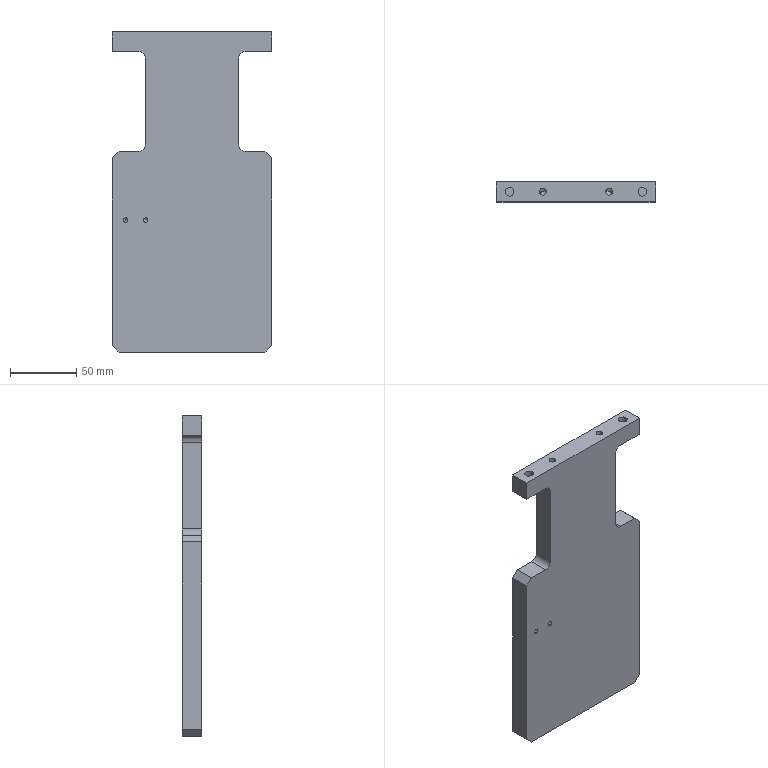Part | STEP file | PN_0048 | 1 solid | 58 faces | box 120 x 15 x 241.5 mm | volume 375920 mm3 | cylinder 24 | plane 18 | cone 16 | commonest cylinder face diameters 3.3 x4 4 x4 4.2 x4 5 x4 6.5 x4 10 x4